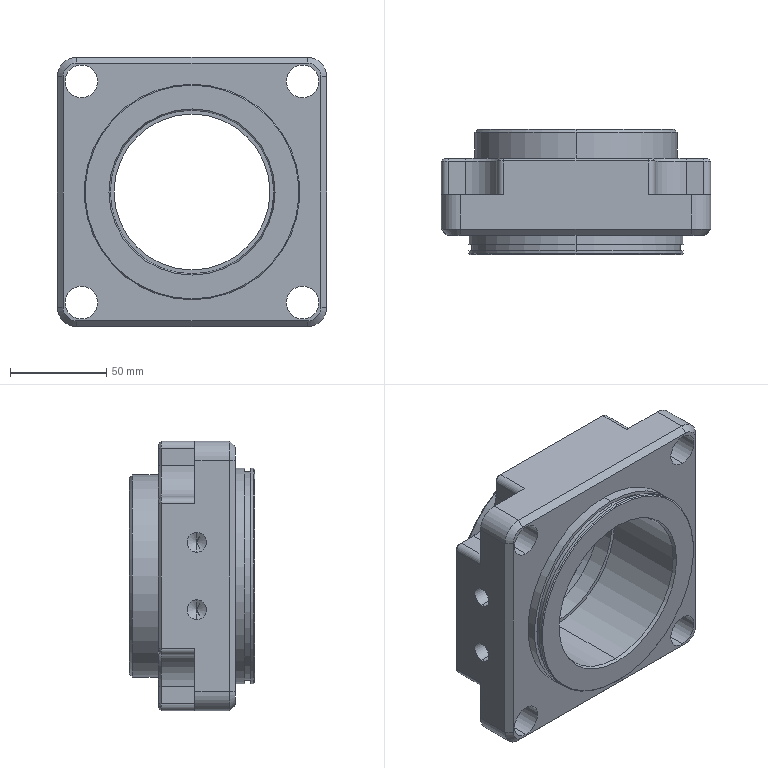Part | SolidWorks | features ICE 12, HoleWzd 11, Chamfer 7, Fillet 4, CirPattern 3, Extrusion 1, MirrorPattern 1, MoveFace 1, RevCut 1 | 1 solid | 153 faces | box 140 x 65 x 140 mm | volume 538697 mm3 | cylinder 64 | cone 48 | plane 41 | commonest cylinder face diameters 8.5 x16 7 x8 10.2 x8 17 x8 20 x4 33 x4